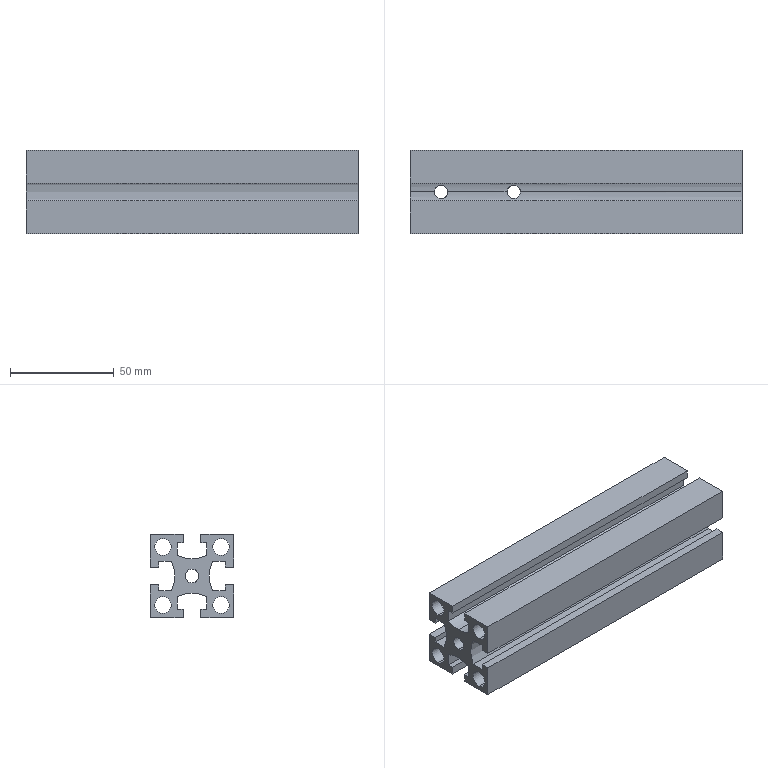Part | STEP file | PN_0071 (reinforcing stop) | 1 solid | 57 faces | box 160 x 40 x 40 mm | volume 131462 mm3 | plane 34 | cylinder 23 | commonest cylinder face diameters 6.5 x8 8 x8 30 x5 6.7 x2